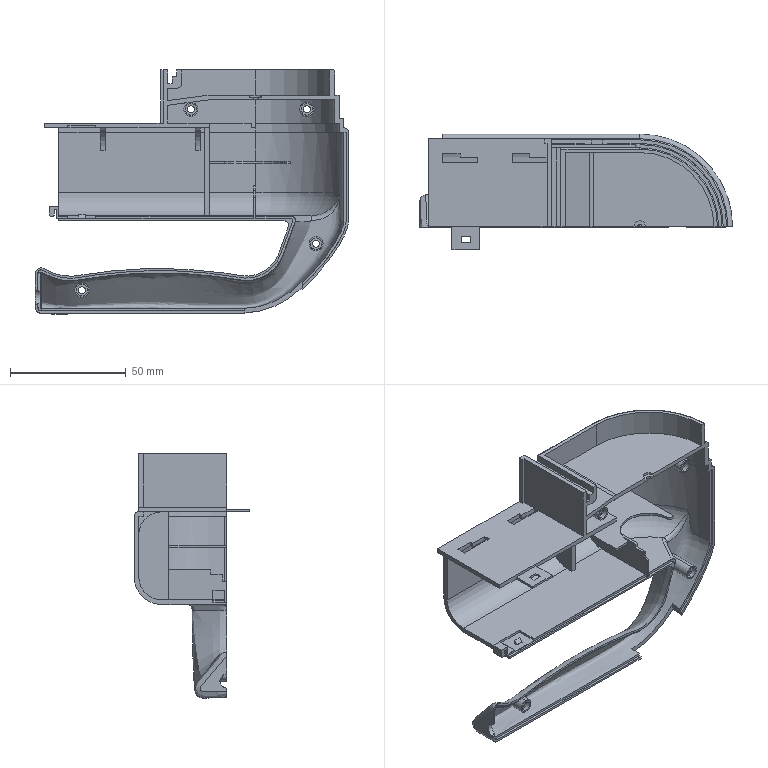Part | SolidWorks | features ICE 24, Fillet 8, BossThin 4, CombineBodies 2, Rib 2, CompositeCurve 1, SewRefSurface 1, Shell 1, Stock 1, SurfCut 1, SweepCut 1 | 2 solids | 269 faces | box 135 x 49.981 x 105.415 mm | volume 48344 mm3 | plane 166 | cylinder 58 | spline 27 | cone 12 | torus 6 | commonest cylinder face diameters 5 x9 6 x9 1 x8 3 x8 20 x5 2 x4